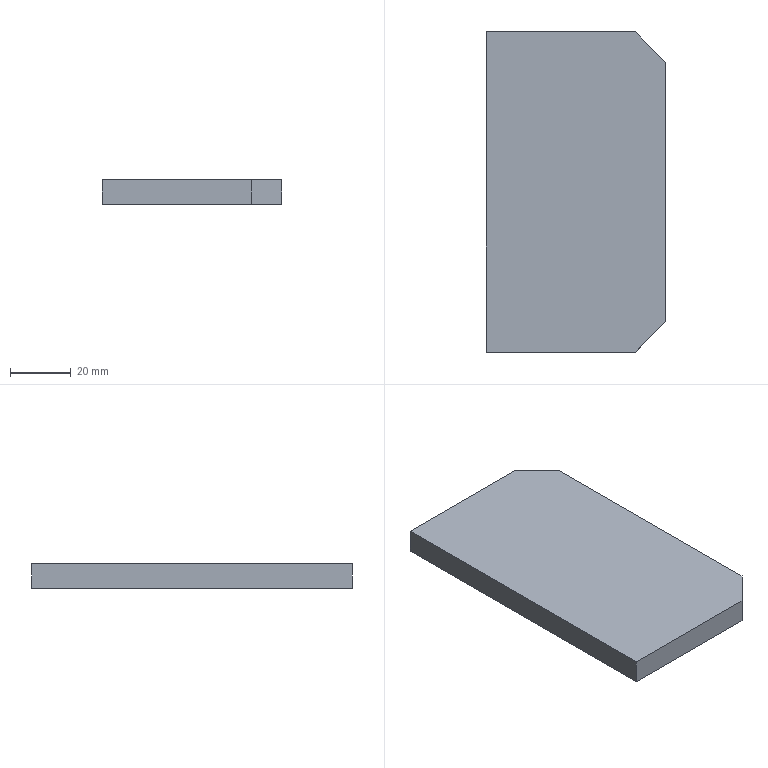Part | STEP file | 08-Rib plate | 1 solid | 8 faces | box 59 x 105 x 8 mm | volume 48760 mm3 | plane 8
STEP:
#1=CARTESIAN_POINT('',(0.,0.,0.));
#2=DIRECTION('',(0.,0.,1.));
#3=DIRECTION('',(1.,0.,0.));
#4=AXIS2_PLACEMENT_3D('',#1,#2,#3);
#5=CARTESIAN_POINT('',(0.,0.,0.));
#6=VERTEX_POINT('',#5);
#7=CARTESIAN_POINT('',(0.,-105.,0.));
#8=VERTEX_POINT('',#7);
#9=CARTESIAN_POINT('',(0.,0.,0.));
#10=DIRECTION('',(0.,-1.,0.));
#11=VECTOR('',#10,1.);
#12=LINE('',#9,#11);
#13=CARTESIAN_POINT('',(0.,0.,8.));
#14=DIRECTION('',(1.,0.,0.));
#15=DIRECTION('',(0.,1.,0.));
#16=AXIS2_PLACEMENT_3D('',#13,#14,#15);
#17=PLANE('',#16);
#18=CARTESIAN_POINT('',(0.,-8.));
#19=DIRECTION('',(-1.,0.));
#20=VECTOR('',#19,1.);
#21=LINE('',#18,#20);
#22=(GEOMETRIC_REPRESENTATION_CONTEXT(2)PARAMETRIC_REPRESENTATION_CONTEXT()REPRESENTATION_CONTEXT('',''));
#23=DEFINITIONAL_REPRESENTATION('',(#21),#22);
#24=PCURVE('',#17,#23);
#25=CARTESIAN_POINT('',(0.,0.,0.));
#26=DIRECTION('',(0.,0.,1.));
#27=DIRECTION('',(1.,0.,0.));
#28=AXIS2_PLACEMENT_3D('',#25,#26,#27);
#29=PLANE('',#28);
#30=CARTESIAN_POINT('',(0.,0.));
#31=DIRECTION('',(0.,-1.));
#32=VECTOR('',#31,1.);
#33=LINE('',#30,#32);
#34=(GEOMETRIC_REPRESENTATION_CONTEXT(2)PARAMETRIC_REPRESENTATION_CONTEXT()REPRESENTATION_CONTEXT('',''));
#35=DEFINITIONAL_REPRESENTATION('',(#33),#34);
#36=PCURVE('',#29,#35);
#37=SURFACE_CURVE('',#12,(#24,#36),.PCURVE_S1.);
#38=EDGE_CURVE('',#6,#8,#37,.T.);
#39=ORIENTED_EDGE('',*,*,#38,.T.);
#40=CARTESIAN_POINT('',(0.,-105.,8.));
#41=VERTEX_POINT('',#40);
#42=CARTESIAN_POINT('',(0.,-105.,8.));
#43=DIRECTION('',(0.,0.,-1.));
#44=VECTOR('',#43,1.);
#45=LINE('',#42,#44);
#46=CARTESIAN_POINT('',(-105.,0.));
#47=DIRECTION('',(0.,-1.));
#48=VECTOR('',#47,1.);
#49=LINE('',#46,#48);
#50=(GEOMETRIC_REPRESENTATION_CONTEXT(2)PARAMETRIC_REPRESENTATION_CONTEXT()REPRESENTATION_CONTEXT('',''));
#51=DEFINITIONAL_REPRESENTATION('',(#49),#50);
#52=PCURVE('',#17,#51);
#53=CARTESIAN_POINT('',(0.,-105.,8.));
#54=DIRECTION('',(0.,1.,0.));
#55=DIRECTION('',(0.,0.,1.));
#56=AXIS2_PLACEMENT_3D('',#53,#54,#55);
#57=PLANE('',#56);
#58=CARTESIAN_POINT('',(0.,0.));
#59=DIRECTION('',(-1.,0.));
#60=VECTOR('',#59,1.);
#61=LINE('',#58,#60);
#62=(GEOMETRIC_REPRESENTATION_CONTEXT(2)PARAMETRIC_REPRESENTATION_CONTEXT()REPRESENTATION_CONTEXT('',''));
#63=DEFINITIONAL_REPRESENTATION('',(#61),#62);
#64=PCURVE('',#57,#63);
#65=SURFACE_CURVE('',#45,(#52,#64),.PCURVE_S1.);
#66=EDGE_CURVE('',#41,#8,#65,.T.);
#67=ORIENTED_EDGE('',*,*,#66,.F.);
#68=CARTESIAN_POINT('',(0.,0.,8.));
#69=VERTEX_POINT('',#68);
#70=CARTESIAN_POINT('',(0.,0.,8.));
#71=DIRECTION('',(0.,-1.,0.));
#72=VECTOR('',#71,1.);
#73=LINE('',#70,#72);
#74=CARTESIAN_POINT('',(0.,0.));
#75=DIRECTION('',(-1.,0.));
#76=VECTOR('',#75,1.);
#77=LINE('',#74,#76);
#78=(GEOMETRIC_REPRESENTATION_CONTEXT(2)PARAMETRIC_REPRESENTATION_CONTEXT()REPRESENTATION_CONTEXT('',''));
#79=DEFINITIONAL_REPRESENTATION('',(#77),#78);
#80=PCURVE('',#17,#79);
#81=CARTESIAN_POINT('',(0.,0.,8.));
#82=DIRECTION('',(0.,0.,1.));
#83=DIRECTION('',(1.,0.,0.));
#84=AXIS2_PLACEMENT_3D('',#81,#82,#83);
#85=PLANE('',#84);
#86=CARTESIAN_POINT('',(0.,0.));
#87=DIRECTION('',(0.,-1.));
#88=VECTOR('',#87,1.);
#89=LINE('',#86,#88);
#90=(GEOMETRIC_REPRESENTATION_CONTEXT(2)PARAMETRIC_REPRESENTATION_CONTEXT()REPRESENTATION_CONTEXT('',''));
#91=DEFINITIONAL_REPRESENTATION('',(#89),#90);
#92=PCURVE('',#85,#91);
#93=SURFACE_CURVE('',#73,(#80,#92),.PCURVE_S1.);
#94=EDGE_CURVE('',#69,#41,#93,.T.);
#95=ORIENTED_EDGE('',*,*,#94,.F.);
#96=CARTESIAN_POINT('',(0.,0.,8.));
#97=DIRECTION('',(0.,0.,-1.));
#98=VECTOR('',#97,1.);
#99=LINE('',#96,#98);
#100=CARTESIAN_POINT('',(0.,0.));
#101=DIRECTION('',(0.,-1.));
#102=VECTOR('',#101,1.);
#103=LINE('',#100,#102);
#104=(GEOMETRIC_REPRESENTATION_CONTEXT(2)PARAMETRIC_REPRESENTATION_CONTEXT()REPRESENTATION_CONTEXT('',''));
#105=DEFINITIONAL_REPRESENTATION('',(#103),#104);
#106=PCURVE('',#17,#105);
#107=CARTESIAN_POINT('',(0.,0.,8.));
#108=DIRECTION('',(0.,-1.,0.));
#109=DIRECTION('',(0.,0.,-1.));
#110=AXIS2_PLACEMENT_3D('',#107,#108,#109);
#111=PLANE('',#110);
#112=CARTESIAN_POINT('',(0.,0.));
#113=DIRECTION('',(1.,0.));
#114=VECTOR('',#113,1.);
#115=LINE('',#112,#114);
#116=(GEOMETRIC_REPRESENTATION_CONTEXT(2)PARAMETRIC_REPRESENTATION_CONTEXT()REPRESENTATION_CONTEXT('',''));
#117=DEFINITIONAL_REPRESENTATION('',(#115),#116);
#118=PCURVE('',#111,#117);
#119=SURFACE_CURVE('',#99,(#106,#118),.PCURVE_S1.);
#120=EDGE_CURVE('',#69,#6,#119,.T.);
#121=ORIENTED_EDGE('',*,*,#120,.T.);
#122=EDGE_LOOP('',(#39,#67,#95,#121));
#123=FACE_BOUND('',#122,.T.);
#124=ADVANCED_FACE('',(#123),#17,.F.);
#125=CARTESIAN_POINT('',(49.,-105.,0.));
#126=VERTEX_POINT('',#125);
#127=CARTESIAN_POINT('',(0.,-105.,0.));
#128=DIRECTION('',(1.,0.,0.));
#129=VECTOR('',#128,1.);
#130=LINE('',#127,#129);
#131=CARTESIAN_POINT('',(-8.,0.));
#132=DIRECTION('',(0.,1.));
#133=VECTOR('',#132,1.);
#134=LINE('',#131,#133);
#135=(GEOMETRIC_REPRESENTATION_CONTEXT(2)PARAMETRIC_REPRESENTATION_CONTEXT()REPRESENTATION_CONTEXT('',''));
#136=DEFINITIONAL_REPRESENTATION('',(#134),#135);
#137=PCURVE('',#57,#136);
#138=CARTESIAN_POINT('',(0.,-105.));
#139=DIRECTION('',(1.,0.));
#140=VECTOR('',#139,1.);
#141=LINE('',#138,#140);
#142=(GEOMETRIC_REPRESENTATION_CONTEXT(2)PARAMETRIC_REPRESENTATION_CONTEXT()REPRESENTATION_CONTEXT('',''));
#143=DEFINITIONAL_REPRESENTATION('',(#141),#142);
#144=PCURVE('',#29,#143);
#145=SURFACE_CURVE('',#130,(#137,#144),.PCURVE_S1.);
#146=EDGE_CURVE('',#8,#126,#145,.T.);
#147=ORIENTED_EDGE('',*,*,#146,.T.);
#148=CARTESIAN_POINT('',(49.,-105.,8.));
#149=VERTEX_POINT('',#148);
#150=CARTESIAN_POINT('',(49.,-105.,8.));
#151=DIRECTION('',(0.,0.,-1.));
#152=VECTOR('',#151,1.);
#153=LINE('',#150,#152);
#154=CARTESIAN_POINT('',(0.,49.));
#155=DIRECTION('',(-1.,0.));
#156=VECTOR('',#155,1.);
#157=LINE('',#154,#156);
#158=(GEOMETRIC_REPRESENTATION_CONTEXT(2)PARAMETRIC_REPRESENTATION_CONTEXT()REPRESENTATION_CONTEXT('',''));
#159=DEFINITIONAL_REPRESENTATION('',(#157),#158);
#160=PCURVE('',#57,#159);
#161=CARTESIAN_POINT('',(59.,-95.,8.));
#162=DIRECTION('',(-0.7071,0.7071,0.));
#163=DIRECTION('',(-0.7071,-0.7071,0.));
#164=AXIS2_PLACEMENT_3D('',#161,#162,#163);
#165=PLANE('',#164);
#166=CARTESIAN_POINT('',(14.142,0.));
#167=DIRECTION('',(0.,-1.));
#168=VECTOR('',#167,1.);
#169=LINE('',#166,#168);
#170=(GEOMETRIC_REPRESENTATION_CONTEXT(2)PARAMETRIC_REPRESENTATION_CONTEXT()REPRESENTATION_CONTEXT('',''));
#171=DEFINITIONAL_REPRESENTATION('',(#169),#170);
#172=PCURVE('',#165,#171);
#173=SURFACE_CURVE('',#153,(#160,#172),.PCURVE_S1.);
#174=EDGE_CURVE('',#149,#126,#173,.T.);
#175=ORIENTED_EDGE('',*,*,#174,.F.);
#176=CARTESIAN_POINT('',(0.,-105.,8.));
#177=DIRECTION('',(1.,0.,0.));
#178=VECTOR('',#177,1.);
#179=LINE('',#176,#178);
#180=CARTESIAN_POINT('',(0.,0.));
#181=DIRECTION('',(0.,1.));
#182=VECTOR('',#181,1.);
#183=LINE('',#180,#182);
#184=(GEOMETRIC_REPRESENTATION_CONTEXT(2)PARAMETRIC_REPRESENTATION_CONTEXT()REPRESENTATION_CONTEXT('',''));
#185=DEFINITIONAL_REPRESENTATION('',(#183),#184);
#186=PCURVE('',#57,#185);
#187=CARTESIAN_POINT('',(0.,-105.));
#188=DIRECTION('',(1.,0.));
#189=VECTOR('',#188,1.);
#190=LINE('',#187,#189);
#191=(GEOMETRIC_REPRESENTATION_CONTEXT(2)PARAMETRIC_REPRESENTATION_CONTEXT()REPRESENTATION_CONTEXT('',''));
#192=DEFINITIONAL_REPRESENTATION('',(#190),#191);
#193=PCURVE('',#85,#192);
#194=SURFACE_CURVE('',#179,(#186,#193),.PCURVE_S1.);
#195=EDGE_CURVE('',#41,#149,#194,.T.);
#196=ORIENTED_EDGE('',*,*,#195,.F.);
#197=ORIENTED_EDGE('',*,*,#66,.T.);
#198=EDGE_LOOP('',(#147,#175,#196,#197));
#199=FACE_BOUND('',#198,.T.);
#200=ADVANCED_FACE('',(#199),#57,.F.);
#201=CARTESIAN_POINT('',(59.,-95.,0.));
#202=VERTEX_POINT('',#201);
#203=CARTESIAN_POINT('',(59.,-95.,0.));
#204=DIRECTION('',(0.7071,0.7071,0.));
#205=VECTOR('',#204,1.);
#206=LINE('',#203,#205);
#207=CARTESIAN_POINT('',(0.,-8.));
#208=DIRECTION('',(-1.,0.));
#209=VECTOR('',#208,1.);
#210=LINE('',#207,#209);
#211=(GEOMETRIC_REPRESENTATION_CONTEXT(2)PARAMETRIC_REPRESENTATION_CONTEXT()REPRESENTATION_CONTEXT('',''));
#212=DEFINITIONAL_REPRESENTATION('',(#210),#211);
#213=PCURVE('',#165,#212);
#214=CARTESIAN_POINT('',(59.,-95.));
#215=DIRECTION('',(0.7071,0.7071));
#216=VECTOR('',#215,1.);
#217=LINE('',#214,#216);
#218=(GEOMETRIC_REPRESENTATION_CONTEXT(2)PARAMETRIC_REPRESENTATION_CONTEXT()REPRESENTATION_CONTEXT('',''));
#219=DEFINITIONAL_REPRESENTATION('',(#217),#218);
#220=PCURVE('',#29,#219);
#221=SURFACE_CURVE('',#206,(#213,#220),.PCURVE_S1.);
#222=EDGE_CURVE('',#126,#202,#221,.T.);
#223=ORIENTED_EDGE('',*,*,#222,.T.);
#224=CARTESIAN_POINT('',(59.,-95.,8.));
#225=VERTEX_POINT('',#224);
#226=CARTESIAN_POINT('',(59.,-95.,8.));
#227=DIRECTION('',(0.,0.,-1.));
#228=VECTOR('',#227,1.);
#229=LINE('',#226,#228);
#230=CARTESIAN_POINT('',(0.,0.));
#231=DIRECTION('',(0.,-1.));
#232=VECTOR('',#231,1.);
#233=LINE('',#230,#232);
#234=(GEOMETRIC_REPRESENTATION_CONTEXT(2)PARAMETRIC_REPRESENTATION_CONTEXT()REPRESENTATION_CONTEXT('',''));
#235=DEFINITIONAL_REPRESENTATION('',(#233),#234);
#236=PCURVE('',#165,#235);
#237=CARTESIAN_POINT('',(59.,-10.,8.));
#238=DIRECTION('',(-1.,0.,0.));
#239=DIRECTION('',(0.,-1.,0.));
#240=AXIS2_PLACEMENT_3D('',#237,#238,#239);
#241=PLANE('',#240);
#242=CARTESIAN_POINT('',(85.,0.));
#243=DIRECTION('',(0.,-1.));
#244=VECTOR('',#243,1.);
#245=LINE('',#242,#244);
#246=(GEOMETRIC_REPRESENTATION_CONTEXT(2)PARAMETRIC_REPRESENTATION_CONTEXT()REPRESENTATION_CONTEXT('',''));
#247=DEFINITIONAL_REPRESENTATION('',(#245),#246);
#248=PCURVE('',#241,#247);
#249=SURFACE_CURVE('',#229,(#236,#248),.PCURVE_S1.);
#250=EDGE_CURVE('',#225,#202,#249,.T.);
#251=ORIENTED_EDGE('',*,*,#250,.F.);
#252=CARTESIAN_POINT('',(59.,-95.,8.));
#253=DIRECTION('',(0.7071,0.7071,0.));
#254=VECTOR('',#253,1.);
#255=LINE('',#252,#254);
#256=CARTESIAN_POINT('',(0.,0.));
#257=DIRECTION('',(-1.,0.));
#258=VECTOR('',#257,1.);
#259=LINE('',#256,#258);
#260=(GEOMETRIC_REPRESENTATION_CONTEXT(2)PARAMETRIC_REPRESENTATION_CONTEXT()REPRESENTATION_CONTEXT('',''));
#261=DEFINITIONAL_REPRESENTATION('',(#259),#260);
#262=PCURVE('',#165,#261);
#263=CARTESIAN_POINT('',(59.,-95.));
#264=DIRECTION('',(0.7071,0.7071));
#265=VECTOR('',#264,1.);
#266=LINE('',#263,#265);
#267=(GEOMETRIC_REPRESENTATION_CONTEXT(2)PARAMETRIC_REPRESENTATION_CONTEXT()REPRESENTATION_CONTEXT('',''));
#268=DEFINITIONAL_REPRESENTATION('',(#266),#267);
#269=PCURVE('',#85,#268);
#270=SURFACE_CURVE('',#255,(#262,#269),.PCURVE_S1.);
#271=EDGE_CURVE('',#149,#225,#270,.T.);
#272=ORIENTED_EDGE('',*,*,#271,.F.);
#273=ORIENTED_EDGE('',*,*,#174,.T.);
#274=EDGE_LOOP('',(#223,#251,#272,#273));
#275=FACE_BOUND('',#274,.T.);
#276=ADVANCED_FACE('',(#275),#165,.F.);
#277=CARTESIAN_POINT('',(59.,-10.,0.));
#278=VERTEX_POINT('',#277);
#279=CARTESIAN_POINT('',(59.,-10.,0.));
#280=DIRECTION('',(0.,1.,0.));
#281=VECTOR('',#280,1.);
#282=LINE('',#279,#281);
#283=CARTESIAN_POINT('',(0.,-8.));
#284=DIRECTION('',(-1.,0.));
#285=VECTOR('',#284,1.);
#286=LINE('',#283,#285);
#287=(GEOMETRIC_REPRESENTATION_CONTEXT(2)PARAMETRIC_REPRESENTATION_CONTEXT()REPRESENTATION_CONTEXT('',''));
#288=DEFINITIONAL_REPRESENTATION('',(#286),#287);
#289=PCURVE('',#241,#288);
#290=CARTESIAN_POINT('',(59.,-10.));
#291=DIRECTION('',(0.,1.));
#292=VECTOR('',#291,1.);
#293=LINE('',#290,#292);
#294=(GEOMETRIC_REPRESENTATION_CONTEXT(2)PARAMETRIC_REPRESENTATION_CONTEXT()REPRESENTATION_CONTEXT('',''));
#295=DEFINITIONAL_REPRESENTATION('',(#293),#294);
#296=PCURVE('',#29,#295);
#297=SURFACE_CURVE('',#282,(#289,#296),.PCURVE_S1.);
#298=EDGE_CURVE('',#202,#278,#297,.T.);
#299=ORIENTED_EDGE('',*,*,#298,.T.);
#300=CARTESIAN_POINT('',(59.,-10.,8.));
#301=VERTEX_POINT('',#300);
#302=CARTESIAN_POINT('',(59.,-10.,8.));
#303=DIRECTION('',(0.,0.,-1.));
#304=VECTOR('',#303,1.);
#305=LINE('',#302,#304);
#306=CARTESIAN_POINT('',(0.,0.));
#307=DIRECTION('',(0.,-1.));
#308=VECTOR('',#307,1.);
#309=LINE('',#306,#308);
#310=(GEOMETRIC_REPRESENTATION_CONTEXT(2)PARAMETRIC_REPRESENTATION_CONTEXT()REPRESENTATION_CONTEXT('',''));
#311=DEFINITIONAL_REPRESENTATION('',(#309),#310);
#312=PCURVE('',#241,#311);
#313=CARTESIAN_POINT('',(49.,0.,8.));
#314=DIRECTION('',(-0.7071,-0.7071,0.));
#315=DIRECTION('',(0.7071,-0.7071,0.));
#316=AXIS2_PLACEMENT_3D('',#313,#314,#315);
#317=PLANE('',#316);
#318=CARTESIAN_POINT('',(14.142,0.));
#319=DIRECTION('',(0.,-1.));
#320=VECTOR('',#319,1.);
#321=LINE('',#318,#320);
#322=(GEOMETRIC_REPRESENTATION_CONTEXT(2)PARAMETRIC_REPRESENTATION_CONTEXT()REPRESENTATION_CONTEXT('',''));
#323=DEFINITIONAL_REPRESENTATION('',(#321),#322);
#324=PCURVE('',#317,#323);
#325=SURFACE_CURVE('',#305,(#312,#324),.PCURVE_S1.);
#326=EDGE_CURVE('',#301,#278,#325,.T.);
#327=ORIENTED_EDGE('',*,*,#326,.F.);
#328=CARTESIAN_POINT('',(59.,-10.,8.));
#329=DIRECTION('',(0.,1.,0.));
#330=VECTOR('',#329,1.);
#331=LINE('',#328,#330);
#332=CARTESIAN_POINT('',(0.,0.));
#333=DIRECTION('',(-1.,0.));
#334=VECTOR('',#333,1.);
#335=LINE('',#332,#334);
#336=(GEOMETRIC_REPRESENTATION_CONTEXT(2)PARAMETRIC_REPRESENTATION_CONTEXT()REPRESENTATION_CONTEXT('',''));
#337=DEFINITIONAL_REPRESENTATION('',(#335),#336);
#338=PCURVE('',#241,#337);
#339=CARTESIAN_POINT('',(59.,-10.));
#340=DIRECTION('',(0.,1.));
#341=VECTOR('',#340,1.);
#342=LINE('',#339,#341);
#343=(GEOMETRIC_REPRESENTATION_CONTEXT(2)PARAMETRIC_REPRESENTATION_CONTEXT()REPRESENTATION_CONTEXT('',''));
#344=DEFINITIONAL_REPRESENTATION('',(#342),#343);
#345=PCURVE('',#85,#344);
#346=SURFACE_CURVE('',#331,(#338,#345),.PCURVE_S1.);
#347=EDGE_CURVE('',#225,#301,#346,.T.);
#348=ORIENTED_EDGE('',*,*,#347,.F.);
#349=ORIENTED_EDGE('',*,*,#250,.T.);
#350=EDGE_LOOP('',(#299,#327,#348,#349));
#351=FACE_BOUND('',#350,.T.);
#352=ADVANCED_FACE('',(#351),#241,.F.);
#353=CARTESIAN_POINT('',(49.,0.,0.));
#354=VERTEX_POINT('',#353);
#355=CARTESIAN_POINT('',(49.,0.,0.));
#356=DIRECTION('',(-0.7071,0.7071,0.));
#357=VECTOR('',#356,1.);
#358=LINE('',#355,#357);
#359=CARTESIAN_POINT('',(0.,-8.));
#360=DIRECTION('',(-1.,0.));
#361=VECTOR('',#360,1.);
#362=LINE('',#359,#361);
#363=(GEOMETRIC_REPRESENTATION_CONTEXT(2)PARAMETRIC_REPRESENTATION_CONTEXT()REPRESENTATION_CONTEXT('',''));
#364=DEFINITIONAL_REPRESENTATION('',(#362),#363);
#365=PCURVE('',#317,#364);
#366=CARTESIAN_POINT('',(49.,0.));
#367=DIRECTION('',(-0.7071,0.7071));
#368=VECTOR('',#367,1.);
#369=LINE('',#366,#368);
#370=(GEOMETRIC_REPRESENTATION_CONTEXT(2)PARAMETRIC_REPRESENTATION_CONTEXT()REPRESENTATION_CONTEXT('',''));
#371=DEFINITIONAL_REPRESENTATION('',(#369),#370);
#372=PCURVE('',#29,#371);
#373=SURFACE_CURVE('',#358,(#365,#372),.PCURVE_S1.);
#374=EDGE_CURVE('',#278,#354,#373,.T.);
#375=ORIENTED_EDGE('',*,*,#374,.T.);
#376=CARTESIAN_POINT('',(49.,0.,8.));
#377=VERTEX_POINT('',#376);
#378=CARTESIAN_POINT('',(49.,0.,8.));
#379=DIRECTION('',(0.,0.,-1.));
#380=VECTOR('',#379,1.);
#381=LINE('',#378,#380);
#382=CARTESIAN_POINT('',(0.,0.));
#383=DIRECTION('',(0.,-1.));
#384=VECTOR('',#383,1.);
#385=LINE('',#382,#384);
#386=(GEOMETRIC_REPRESENTATION_CONTEXT(2)PARAMETRIC_REPRESENTATION_CONTEXT()REPRESENTATION_CONTEXT('',''));
#387=DEFINITIONAL_REPRESENTATION('',(#385),#386);
#388=PCURVE('',#317,#387);
#389=CARTESIAN_POINT('',(0.,49.));
#390=DIRECTION('',(1.,0.));
#391=VECTOR('',#390,1.);
#392=LINE('',#389,#391);
#393=(GEOMETRIC_REPRESENTATION_CONTEXT(2)PARAMETRIC_REPRESENTATION_CONTEXT()REPRESENTATION_CONTEXT('',''));
#394=DEFINITIONAL_REPRESENTATION('',(#392),#393);
#395=PCURVE('',#111,#394);
#396=SURFACE_CURVE('',#381,(#388,#395),.PCURVE_S1.);
#397=EDGE_CURVE('',#377,#354,#396,.T.);
#398=ORIENTED_EDGE('',*,*,#397,.F.);
#399=CARTESIAN_POINT('',(49.,0.,8.));
#400=DIRECTION('',(-0.7071,0.7071,0.));
#401=VECTOR('',#400,1.);
#402=LINE('',#399,#401);
#403=CARTESIAN_POINT('',(0.,0.));
#404=DIRECTION('',(-1.,0.));
#405=VECTOR('',#404,1.);
#406=LINE('',#403,#405);
#407=(GEOMETRIC_REPRESENTATION_CONTEXT(2)PARAMETRIC_REPRESENTATION_CONTEXT()REPRESENTATION_CONTEXT('',''));
#408=DEFINITIONAL_REPRESENTATION('',(#406),#407);
#409=PCURVE('',#317,#408);
#410=CARTESIAN_POINT('',(49.,0.));
#411=DIRECTION('',(-0.7071,0.7071));
#412=VECTOR('',#411,1.);
#413=LINE('',#410,#412);
#414=(GEOMETRIC_REPRESENTATION_CONTEXT(2)PARAMETRIC_REPRESENTATION_CONTEXT()REPRESENTATION_CONTEXT('',''));
#415=DEFINITIONAL_REPRESENTATION('',(#413),#414);
#416=PCURVE('',#85,#415);
#417=SURFACE_CURVE('',#402,(#409,#416),.PCURVE_S1.);
#418=EDGE_CURVE('',#301,#377,#417,.T.);
#419=ORIENTED_EDGE('',*,*,#418,.F.);
#420=ORIENTED_EDGE('',*,*,#326,.T.);
#421=EDGE_LOOP('',(#375,#398,#419,#420));
#422=FACE_BOUND('',#421,.T.);
#423=ADVANCED_FACE('',(#422),#317,.F.);
#424=CARTESIAN_POINT('',(0.,0.,0.));
#425=DIRECTION('',(-1.,0.,0.));
#426=VECTOR('',#425,1.);
#427=LINE('',#424,#426);
#428=CARTESIAN_POINT('',(8.,0.));
#429=DIRECTION('',(0.,-1.));
#430=VECTOR('',#429,1.);
#431=LINE('',#428,#430);
#432=(GEOMETRIC_REPRESENTATION_CONTEXT(2)PARAMETRIC_REPRESENTATION_CONTEXT()REPRESENTATION_CONTEXT('',''));
#433=DEFINITIONAL_REPRESENTATION('',(#431),#432);
#434=PCURVE('',#111,#433);
#435=CARTESIAN_POINT('',(0.,0.));
#436=DIRECTION('',(-1.,0.));
#437=VECTOR('',#436,1.);
#438=LINE('',#435,#437);
#439=(GEOMETRIC_REPRESENTATION_CONTEXT(2)PARAMETRIC_REPRESENTATION_CONTEXT()REPRESENTATION_CONTEXT('',''));
#440=DEFINITIONAL_REPRESENTATION('',(#438),#439);
#441=PCURVE('',#29,#440);
#442=SURFACE_CURVE('',#427,(#434,#441),.PCURVE_S1.);
#443=EDGE_CURVE('',#354,#6,#442,.T.);
#444=ORIENTED_EDGE('',*,*,#443,.T.);
#445=ORIENTED_EDGE('',*,*,#120,.F.);
#446=CARTESIAN_POINT('',(0.,0.,8.));
#447=DIRECTION('',(-1.,0.,0.));
#448=VECTOR('',#447,1.);
#449=LINE('',#446,#448);
#450=CARTESIAN_POINT('',(0.,0.));
#451=DIRECTION('',(0.,-1.));
#452=VECTOR('',#451,1.);
#453=LINE('',#450,#452);
#454=(GEOMETRIC_REPRESENTATION_CONTEXT(2)PARAMETRIC_REPRESENTATION_CONTEXT()REPRESENTATION_CONTEXT('',''));
#455=DEFINITIONAL_REPRESENTATION('',(#453),#454);
#456=PCURVE('',#111,#455);
#457=CARTESIAN_POINT('',(0.,0.));
#458=DIRECTION('',(-1.,0.));
#459=VECTOR('',#458,1.);
#460=LINE('',#457,#459);
#461=(GEOMETRIC_REPRESENTATION_CONTEXT(2)PARAMETRIC_REPRESENTATION_CONTEXT()REPRESENTATION_CONTEXT('',''));
#462=DEFINITIONAL_REPRESENTATION('',(#460),#461);
#463=PCURVE('',#85,#462);
#464=SURFACE_CURVE('',#449,(#456,#463),.PCURVE_S1.);
#465=EDGE_CURVE('',#377,#69,#464,.T.);
#466=ORIENTED_EDGE('',*,*,#465,.F.);
#467=ORIENTED_EDGE('',*,*,#397,.T.);
#468=EDGE_LOOP('',(#444,#445,#466,#467));
#469=FACE_BOUND('',#468,.T.);
#470=ADVANCED_FACE('',(#469),#111,.F.);
#471=ORIENTED_EDGE('',*,*,#94,.T.);
#472=ORIENTED_EDGE('',*,*,#195,.T.);
#473=ORIENTED_EDGE('',*,*,#271,.T.);
#474=ORIENTED_EDGE('',*,*,#347,.T.);
#475=ORIENTED_EDGE('',*,*,#418,.T.);
#476=ORIENTED_EDGE('',*,*,#465,.T.);
#477=EDGE_LOOP('',(#471,#472,#473,#474,#475,#476));
#478=FACE_BOUND('',#477,.T.);
#479=ADVANCED_FACE('',(#478),#85,.T.);
#480=ORIENTED_EDGE('',*,*,#38,.F.);
#481=ORIENTED_EDGE('',*,*,#443,.F.);
#482=ORIENTED_EDGE('',*,*,#374,.F.);
#483=ORIENTED_EDGE('',*,*,#298,.F.);
#484=ORIENTED_EDGE('',*,*,#222,.F.);
#485=ORIENTED_EDGE('',*,*,#146,.F.);
#486=EDGE_LOOP('',(#480,#481,#482,#483,#484,#485));
#487=FACE_BOUND('',#486,.T.);
#488=ADVANCED_FACE('',(#487),#29,.F.);
#489=CLOSED_SHELL('',(#124,#200,#276,#352,#423,#470,#479,#488));
#490=MANIFOLD_SOLID_BREP('',#489);
#491=(LENGTH_UNIT()NAMED_UNIT(*)SI_UNIT(.MILLI.,.METRE.));
#492=UNCERTAINTY_MEASURE_WITH_UNIT(LENGTH_MEASURE(0.0000001),#491,'','');
#493=(NAMED_UNIT(*)PLANE_ANGLE_UNIT()SI_UNIT($,.RADIAN.));
#494=(NAMED_UNIT(*)SI_UNIT($,.STERADIAN.)SOLID_ANGLE_UNIT());
#495=(GEOMETRIC_REPRESENTATION_CONTEXT(3)GLOBAL_UNCERTAINTY_ASSIGNED_CONTEXT((#492))GLOBAL_UNIT_ASSIGNED_CONTEXT((#491,#493,#494))REPRESENTATION_CONTEXT('',''));
#496=ADVANCED_BREP_SHAPE_REPRESENTATION('',(#4,#490),#495);